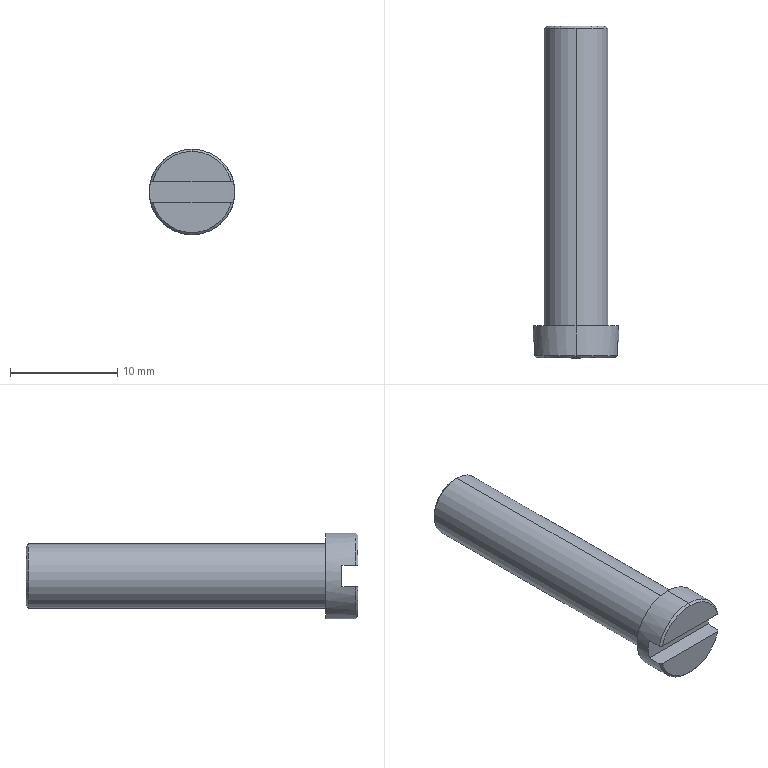Part | NX | features BREP 1 | 1 solid | 20 faces | box 8 x 31 x 8 mm | volume 879.904 mm3 | plane 7 | cone 7 | cylinder 6 | commonest cylinder face diameters 2.5 x2 6 x2 8 x2
STEP:
#1=CARTESIAN_POINT('',(3.873,1.5,1.));
#2=VERTEX_POINT('',#1);
#3=CARTESIAN_POINT('',(-3.873,1.5,1.));
#4=VERTEX_POINT('',#3);
#5=CARTESIAN_POINT('',(-4.,1.5,1.));
#6=DIRECTION('',(-1.,0.,0.));
#7=VECTOR('',#6,1000.);
#8=LINE('',#5,#7);
#9=EDGE_CURVE('',#2,#4,#8,.T.);
#10=ORIENTED_EDGE('',*,*,#9,.T.);
#11=CARTESIAN_POINT('',(-3.873,1.5,-1.));
#12=VERTEX_POINT('',#11);
#13=CARTESIAN_POINT('',(0.,1.5,0.));
#14=DIRECTION('',(0.,-1.,0.));
#15=DIRECTION('',(0.,0.,1.));
#16=AXIS2_PLACEMENT_3D('',#13,#14,#15);
#17=CIRCLE('',#16,4.);
#18=EDGE_CURVE('',#4,#12,#17,.T.);
#19=ORIENTED_EDGE('',*,*,#18,.T.);
#20=CARTESIAN_POINT('',(3.873,1.5,-1.));
#21=VERTEX_POINT('',#20);
#22=CARTESIAN_POINT('',(-4.,1.5,-1.));
#23=DIRECTION('',(1.,0.,0.));
#24=VECTOR('',#23,1000.);
#25=LINE('',#22,#24);
#26=EDGE_CURVE('',#12,#21,#25,.T.);
#27=ORIENTED_EDGE('',*,*,#26,.T.);
#28=CARTESIAN_POINT('',(0.,1.5,0.));
#29=DIRECTION('',(0.,-1.,0.));
#30=DIRECTION('',(0.,0.,1.));
#31=AXIS2_PLACEMENT_3D('',#28,#29,#30);
#32=CIRCLE('',#31,4.);
#33=EDGE_CURVE('',#21,#2,#32,.T.);
#34=ORIENTED_EDGE('',*,*,#33,.T.);
#35=EDGE_LOOP('',(#10,#19,#27,#34));
#36=FACE_BOUND('',#35,.T.);
#37=CARTESIAN_POINT('',(0.,1.5,0.));
#38=DIRECTION('',(0.,1.,0.));
#39=DIRECTION('',(0.,0.,1.));
#40=AXIS2_PLACEMENT_3D('',#37,#38,#39);
#41=PLANE('',#40);
#42=ADVANCED_FACE('',(#36),#41,.F.);
#43=CARTESIAN_POINT('',(3.873,0.2,1.));
#44=VERTEX_POINT('',#43);
#45=CARTESIAN_POINT('',(3.873,0.,1.));
#46=DIRECTION('',(0.,-1.,0.));
#47=VECTOR('',#46,1000.);
#48=LINE('',#45,#47);
#49=EDGE_CURVE('',#2,#44,#48,.T.);
#50=ORIENTED_EDGE('',*,*,#49,.T.);
#51=CARTESIAN_POINT('',(3.666,0.,1.));
#52=VERTEX_POINT('',#51);
#53=CARTESIAN_POINT('',(3.873,0.2,1.));
#54=CARTESIAN_POINT('',(3.804,0.1333,1.));
#55=CARTESIAN_POINT('',(3.735,0.0666,1.));
#56=CARTESIAN_POINT('',(3.666,0.,1.));
#57=B_SPLINE_CURVE_WITH_KNOTS('',3,(#53,#54,#55,#56),.UNSPECIFIED.,.F.,.F.,(4,4),(0.00684,0.007128),.UNSPECIFIED.);
#58=EDGE_CURVE('',#44,#52,#57,.T.);
#59=ORIENTED_EDGE('',*,*,#58,.T.);
#60=CARTESIAN_POINT('',(-3.666,0.,1.));
#61=VERTEX_POINT('',#60);
#62=CARTESIAN_POINT('',(-4.,0.,1.));
#63=DIRECTION('',(-1.,0.,0.));
#64=VECTOR('',#63,1000.);
#65=LINE('',#62,#64);
#66=EDGE_CURVE('',#52,#61,#65,.T.);
#67=ORIENTED_EDGE('',*,*,#66,.T.);
#68=CARTESIAN_POINT('',(-3.873,0.2,1.));
#69=VERTEX_POINT('',#68);
#70=CARTESIAN_POINT('',(-3.666,0.,1.));
#71=CARTESIAN_POINT('',(-3.735,0.0666,1.));
#72=CARTESIAN_POINT('',(-3.804,0.1333,1.));
#73=CARTESIAN_POINT('',(-3.873,0.2,1.));
#74=B_SPLINE_CURVE_WITH_KNOTS('',3,(#70,#71,#72,#73),.UNSPECIFIED.,.F.,.F.,(4,4),(0.01642,0.01671),.UNSPECIFIED.);
#75=EDGE_CURVE('',#61,#69,#74,.T.);
#76=ORIENTED_EDGE('',*,*,#75,.T.);
#77=CARTESIAN_POINT('',(-3.873,0.,1.));
#78=DIRECTION('',(0.,1.,0.));
#79=VECTOR('',#78,1000.);
#80=LINE('',#77,#79);
#81=EDGE_CURVE('',#69,#4,#80,.T.);
#82=ORIENTED_EDGE('',*,*,#81,.T.);
#83=ORIENTED_EDGE('',*,*,#9,.F.);
#84=EDGE_LOOP('',(#50,#59,#67,#76,#82,#83));
#85=FACE_BOUND('',#84,.T.);
#86=CARTESIAN_POINT('',(-4.,1.5,1.));
#87=DIRECTION('',(0.,0.,1.));
#88=DIRECTION('',(1.,0.,0.));
#89=AXIS2_PLACEMENT_3D('',#86,#87,#88);
#90=PLANE('',#89);
#91=ADVANCED_FACE('',(#85),#90,.F.);
#92=CARTESIAN_POINT('',(-3.873,0.2,-1.));
#93=VERTEX_POINT('',#92);
#94=CARTESIAN_POINT('',(-3.873,0.,-1.));
#95=DIRECTION('',(0.,-1.,0.));
#96=VECTOR('',#95,1000.);
#97=LINE('',#94,#96);
#98=EDGE_CURVE('',#12,#93,#97,.T.);
#99=ORIENTED_EDGE('',*,*,#98,.T.);
#100=CARTESIAN_POINT('',(-3.666,0.,-1.));
#101=VERTEX_POINT('',#100);
#102=CARTESIAN_POINT('',(-3.873,0.2,-1.));
#103=CARTESIAN_POINT('',(-3.804,0.1333,-1.));
#104=CARTESIAN_POINT('',(-3.735,0.0666,-1.));
#105=CARTESIAN_POINT('',(-3.666,0.,-1.));
#106=B_SPLINE_CURVE_WITH_KNOTS('',3,(#102,#103,#104,#105),.UNSPECIFIED.,.F.,.F.,(4,4),(0.00684,0.007128),.UNSPECIFIED.);
#107=EDGE_CURVE('',#93,#101,#106,.T.);
#108=ORIENTED_EDGE('',*,*,#107,.T.);
#109=CARTESIAN_POINT('',(3.666,0.,-1.));
#110=VERTEX_POINT('',#109);
#111=CARTESIAN_POINT('',(-4.,0.,-1.));
#112=DIRECTION('',(1.,0.,0.));
#113=VECTOR('',#112,1000.);
#114=LINE('',#111,#113);
#115=EDGE_CURVE('',#101,#110,#114,.T.);
#116=ORIENTED_EDGE('',*,*,#115,.T.);
#117=CARTESIAN_POINT('',(3.873,0.2,-1.));
#118=VERTEX_POINT('',#117);
#119=CARTESIAN_POINT('',(3.666,0.,-1.));
#120=CARTESIAN_POINT('',(3.735,0.0666,-1.));
#121=CARTESIAN_POINT('',(3.804,0.1333,-1.));
#122=CARTESIAN_POINT('',(3.873,0.2,-1.));
#123=B_SPLINE_CURVE_WITH_KNOTS('',3,(#119,#120,#121,#122),.UNSPECIFIED.,.F.,.F.,(4,4),(0.01642,0.01671),.UNSPECIFIED.);
#124=EDGE_CURVE('',#110,#118,#123,.T.);
#125=ORIENTED_EDGE('',*,*,#124,.T.);
#126=CARTESIAN_POINT('',(3.873,0.,-1.));
#127=DIRECTION('',(0.,1.,0.));
#128=VECTOR('',#127,1000.);
#129=LINE('',#126,#128);
#130=EDGE_CURVE('',#118,#21,#129,.T.);
#131=ORIENTED_EDGE('',*,*,#130,.T.);
#132=ORIENTED_EDGE('',*,*,#26,.F.);
#133=EDGE_LOOP('',(#99,#108,#116,#125,#131,#132));
#134=FACE_BOUND('',#133,.T.);
#135=CARTESIAN_POINT('',(-4.,1.5,-1.));
#136=DIRECTION('',(0.,0.,-1.));
#137=DIRECTION('',(-1.,0.,0.));
#138=AXIS2_PLACEMENT_3D('',#135,#136,#137);
#139=PLANE('',#138);
#140=ADVANCED_FACE('',(#134),#139,.F.);
#141=CARTESIAN_POINT('',(0.,0.,3.8));
#142=VERTEX_POINT('',#141);
#143=CARTESIAN_POINT('',(0.,0.2,4.));
#144=VERTEX_POINT('',#143);
#145=CARTESIAN_POINT('',(0.,0.2,4.));
#146=DIRECTION('',(0.,0.7071,0.7071));
#147=VECTOR('',#146,1000.);
#148=LINE('',#145,#147);
#149=EDGE_CURVE('',#142,#144,#148,.T.);
#150=ORIENTED_EDGE('',*,*,#149,.F.);
#151=CARTESIAN_POINT('',(0.,0.,0.));
#152=DIRECTION('',(0.,-1.,0.));
#153=DIRECTION('',(0.,0.,-1.));
#154=AXIS2_PLACEMENT_3D('',#151,#152,#153);
#155=CIRCLE('',#154,3.8);
#156=EDGE_CURVE('',#52,#142,#155,.T.);
#157=ORIENTED_EDGE('',*,*,#156,.F.);
#158=ORIENTED_EDGE('',*,*,#58,.F.);
#159=CARTESIAN_POINT('',(0.,0.2,0.));
#160=DIRECTION('',(0.,1.,0.));
#161=DIRECTION('',(0.,0.,-1.));
#162=AXIS2_PLACEMENT_3D('',#159,#160,#161);
#163=CIRCLE('',#162,4.);
#164=EDGE_CURVE('',#144,#44,#163,.T.);
#165=ORIENTED_EDGE('',*,*,#164,.F.);
#166=EDGE_LOOP('',(#150,#157,#158,#165));
#167=FACE_BOUND('',#166,.T.);
#168=CARTESIAN_POINT('',(0.,0.2,0.));
#169=DIRECTION('',(0.,1.,0.));
#170=DIRECTION('',(0.,0.,1.));
#171=AXIS2_PLACEMENT_3D('',#168,#169,#170);
#172=CONICAL_SURFACE('',#171,4.,0.7854);
#173=ADVANCED_FACE('',(#167),#172,.T.);
#174=CARTESIAN_POINT('',(0.,31.,2.8));
#175=VERTEX_POINT('',#174);
#176=CARTESIAN_POINT('',(0.,30.8,3.));
#177=VERTEX_POINT('',#176);
#178=CARTESIAN_POINT('',(0.,31.,2.8));
#179=DIRECTION('',(0.,-0.7071,0.7071));
#180=VECTOR('',#179,1000.);
#181=LINE('',#178,#180);
#182=EDGE_CURVE('',#175,#177,#181,.T.);
#183=ORIENTED_EDGE('',*,*,#182,.F.);
#184=CARTESIAN_POINT('',(0.,31.,-2.8));
#185=VERTEX_POINT('',#184);
#186=CARTESIAN_POINT('',(0.,31.,0.));
#187=DIRECTION('',(0.,1.,0.));
#188=DIRECTION('',(0.,0.,1.));
#189=AXIS2_PLACEMENT_3D('',#186,#187,#188);
#190=CIRCLE('',#189,2.8);
#191=EDGE_CURVE('',#185,#175,#190,.T.);
#192=ORIENTED_EDGE('',*,*,#191,.F.);
#193=CARTESIAN_POINT('',(0.,30.8,-3.));
#194=VERTEX_POINT('',#193);
#195=CARTESIAN_POINT('',(0.,31.,-2.8));
#196=DIRECTION('',(0.,-0.7071,-0.7071));
#197=VECTOR('',#196,1000.);
#198=LINE('',#195,#197);
#199=EDGE_CURVE('',#185,#194,#198,.T.);
#200=ORIENTED_EDGE('',*,*,#199,.T.);
#201=CARTESIAN_POINT('',(0.,30.8,0.));
#202=DIRECTION('',(0.,-1.,0.));
#203=DIRECTION('',(0.,0.,1.));
#204=AXIS2_PLACEMENT_3D('',#201,#202,#203);
#205=CIRCLE('',#204,3.);
#206=EDGE_CURVE('',#177,#194,#205,.T.);
#207=ORIENTED_EDGE('',*,*,#206,.F.);
#208=EDGE_LOOP('',(#183,#192,#200,#207));
#209=FACE_BOUND('',#208,.T.);
#210=CARTESIAN_POINT('',(0.,31.,0.));
#211=DIRECTION('',(0.,-1.,0.));
#212=DIRECTION('',(0.,0.,-1.));
#213=AXIS2_PLACEMENT_3D('',#210,#211,#212);
#214=CONICAL_SURFACE('',#213,2.8,0.7854);
#215=ADVANCED_FACE('',(#209),#214,.T.);
#216=CARTESIAN_POINT('',(0.,31.,-1.25));
#217=VERTEX_POINT('',#216);
#218=CARTESIAN_POINT('',(0.,23.5,-1.25));
#219=VERTEX_POINT('',#218);
#220=CARTESIAN_POINT('',(0.,31.,-1.25));
#221=DIRECTION('',(0.,1.,0.));
#222=VECTOR('',#221,1000.);
#223=LINE('',#220,#222);
#224=EDGE_CURVE('',#217,#219,#223,.F.);
#225=ORIENTED_EDGE('',*,*,#224,.T.);
#226=CARTESIAN_POINT('',(0.,23.5,1.25));
#227=VERTEX_POINT('',#226);
#228=CARTESIAN_POINT('',(0.,23.5,0.));
#229=DIRECTION('',(0.,1.,0.));
#230=DIRECTION('',(0.,0.,1.));
#231=AXIS2_PLACEMENT_3D('',#228,#229,#230);
#232=CIRCLE('',#231,1.25);
#233=EDGE_CURVE('',#227,#219,#232,.T.);
#234=ORIENTED_EDGE('',*,*,#233,.F.);
#235=CARTESIAN_POINT('',(0.,31.,1.25));
#236=VERTEX_POINT('',#235);
#237=CARTESIAN_POINT('',(0.,31.,1.25));
#238=DIRECTION('',(0.,1.,0.));
#239=VECTOR('',#238,1000.);
#240=LINE('',#237,#239);
#241=EDGE_CURVE('',#236,#227,#240,.F.);
#242=ORIENTED_EDGE('',*,*,#241,.F.);
#243=CARTESIAN_POINT('',(0.,31.,0.));
#244=DIRECTION('',(0.,1.,0.));
#245=DIRECTION('',(0.,0.,1.));
#246=AXIS2_PLACEMENT_3D('',#243,#244,#245);
#247=CIRCLE('',#246,1.25);
#248=EDGE_CURVE('',#236,#217,#247,.T.);
#249=ORIENTED_EDGE('',*,*,#248,.T.);
#250=EDGE_LOOP('',(#225,#234,#242,#249));
#251=FACE_BOUND('',#250,.T.);
#252=CARTESIAN_POINT('',(0.,31.,0.));
#253=DIRECTION('',(0.,1.,0.));
#254=DIRECTION('',(0.,0.,1.));
#255=AXIS2_PLACEMENT_3D('',#252,#253,#254);
#256=CYLINDRICAL_SURFACE('',#255,1.25);
#257=ADVANCED_FACE('',(#251),#256,.F.);
#258=CARTESIAN_POINT('',(0.,22.749,0.));
#259=VERTEX_POINT('',#258);
#260=CARTESIAN_POINT('',(0.,23.5,-1.25));
#261=DIRECTION('',(0.,0.515,-0.8572));
#262=VECTOR('',#261,1000.);
#263=LINE('',#260,#262);
#264=EDGE_CURVE('',#259,#219,#263,.T.);
#265=ORIENTED_EDGE('',*,*,#264,.F.);
#266=CARTESIAN_POINT('',(0.,23.5,1.25));
#267=DIRECTION('',(0.,0.515,0.8572));
#268=VECTOR('',#267,1000.);
#269=LINE('',#266,#268);
#270=EDGE_CURVE('',#259,#227,#269,.T.);
#271=ORIENTED_EDGE('',*,*,#270,.T.);
#272=ORIENTED_EDGE('',*,*,#233,.T.);
#273=EDGE_LOOP('',(#265,#271,#272));
#274=FACE_BOUND('',#273,.T.);
#275=CARTESIAN_POINT('',(0.,23.5,0.));
#276=DIRECTION('',(0.,1.,0.));
#277=DIRECTION('',(0.,0.,1.));
#278=AXIS2_PLACEMENT_3D('',#275,#276,#277);
#279=CONICAL_SURFACE('',#278,1.25,1.03);
#280=ADVANCED_FACE('',(#274),#279,.F.);
#281=ORIENTED_EDGE('',*,*,#66,.F.);
#282=ORIENTED_EDGE('',*,*,#156,.T.);
#283=CARTESIAN_POINT('',(0.,0.,0.));
#284=DIRECTION('',(0.,-1.,0.));
#285=DIRECTION('',(0.,0.,-1.));
#286=AXIS2_PLACEMENT_3D('',#283,#284,#285);
#287=CIRCLE('',#286,3.8);
#288=EDGE_CURVE('',#142,#61,#287,.T.);
#289=ORIENTED_EDGE('',*,*,#288,.T.);
#290=EDGE_LOOP('',(#281,#282,#289));
#291=FACE_BOUND('',#290,.T.);
#292=CARTESIAN_POINT('',(0.,0.,0.));
#293=DIRECTION('',(0.,-1.,0.));
#294=DIRECTION('',(0.,0.,-1.));
#295=AXIS2_PLACEMENT_3D('',#292,#293,#294);
#296=PLANE('',#295);
#297=ADVANCED_FACE('',(#291),#296,.T.);
#298=CARTESIAN_POINT('',(0.,3.,-4.));
#299=VERTEX_POINT('',#298);
#300=CARTESIAN_POINT('',(0.,0.2,-4.));
#301=VERTEX_POINT('',#300);
#302=CARTESIAN_POINT('',(0.,0.,-4.));
#303=DIRECTION('',(0.,1.,0.));
#304=VECTOR('',#303,1000.);
#305=LINE('',#302,#304);
#306=EDGE_CURVE('',#299,#301,#305,.F.);
#307=ORIENTED_EDGE('',*,*,#306,.T.);
#308=CARTESIAN_POINT('',(0.,0.2,0.));
#309=DIRECTION('',(0.,1.,0.));
#310=DIRECTION('',(0.,0.,-1.));
#311=AXIS2_PLACEMENT_3D('',#308,#309,#310);
#312=CIRCLE('',#311,4.);
#313=EDGE_CURVE('',#301,#93,#312,.T.);
#314=ORIENTED_EDGE('',*,*,#313,.T.);
#315=ORIENTED_EDGE('',*,*,#98,.F.);
#316=ORIENTED_EDGE('',*,*,#18,.F.);
#317=ORIENTED_EDGE('',*,*,#81,.F.);
#318=CARTESIAN_POINT('',(0.,0.2,0.));
#319=DIRECTION('',(0.,1.,0.));
#320=DIRECTION('',(0.,0.,-1.));
#321=AXIS2_PLACEMENT_3D('',#318,#319,#320);
#322=CIRCLE('',#321,4.);
#323=EDGE_CURVE('',#69,#144,#322,.T.);
#324=ORIENTED_EDGE('',*,*,#323,.T.);
#325=CARTESIAN_POINT('',(0.,3.,4.));
#326=VERTEX_POINT('',#325);
#327=CARTESIAN_POINT('',(0.,0.,4.));
#328=DIRECTION('',(0.,1.,0.));
#329=VECTOR('',#328,1000.);
#330=LINE('',#327,#329);
#331=EDGE_CURVE('',#326,#144,#330,.F.);
#332=ORIENTED_EDGE('',*,*,#331,.F.);
#333=CARTESIAN_POINT('',(0.,3.,0.));
#334=DIRECTION('',(0.,1.,0.));
#335=DIRECTION('',(0.,0.,1.));
#336=AXIS2_PLACEMENT_3D('',#333,#334,#335);
#337=CIRCLE('',#336,4.);
#338=EDGE_CURVE('',#299,#326,#337,.T.);
#339=ORIENTED_EDGE('',*,*,#338,.F.);
#340=EDGE_LOOP('',(#307,#314,#315,#316,#317,#324,#332,#339));
#341=FACE_BOUND('',#340,.T.);
#342=CARTESIAN_POINT('',(0.,0.,0.));
#343=DIRECTION('',(0.,1.,0.));
#344=DIRECTION('',(0.,0.,1.));
#345=AXIS2_PLACEMENT_3D('',#342,#343,#344);
#346=CYLINDRICAL_SURFACE('',#345,4.);
#347=ADVANCED_FACE('',(#341),#346,.T.);
#348=CARTESIAN_POINT('',(0.,3.,3.));
#349=VERTEX_POINT('',#348);
#350=CARTESIAN_POINT('',(0.,3.,-3.));
#351=VERTEX_POINT('',#350);
#352=CARTESIAN_POINT('',(0.,3.,0.));
#353=DIRECTION('',(0.,1.,0.));
#354=DIRECTION('',(0.,0.,1.));
#355=AXIS2_PLACEMENT_3D('',#352,#353,#354);
#356=CIRCLE('',#355,3.);
#357=EDGE_CURVE('',#349,#351,#356,.T.);
#358=ORIENTED_EDGE('',*,*,#357,.F.);
#359=CARTESIAN_POINT('',(0.,3.,0.));
#360=DIRECTION('',(0.,1.,0.));
#361=DIRECTION('',(0.,0.,1.));
#362=AXIS2_PLACEMENT_3D('',#359,#360,#361);
#363=CIRCLE('',#362,3.);
#364=EDGE_CURVE('',#351,#349,#363,.T.);
#365=ORIENTED_EDGE('',*,*,#364,.F.);
#366=EDGE_LOOP('',(#358,#365));
#367=FACE_BOUND('',#366,.T.);
#368=CARTESIAN_POINT('',(0.,3.,0.));
#369=DIRECTION('',(0.,1.,0.));
#370=DIRECTION('',(0.,0.,1.));
#371=AXIS2_PLACEMENT_3D('',#368,#369,#370);
#372=CIRCLE('',#371,4.);
#373=EDGE_CURVE('',#326,#299,#372,.T.);
#374=ORIENTED_EDGE('',*,*,#373,.T.);
#375=ORIENTED_EDGE('',*,*,#338,.T.);
#376=EDGE_LOOP('',(#374,#375));
#377=FACE_BOUND('',#376,.T.);
#378=CARTESIAN_POINT('',(0.,3.,0.));
#379=DIRECTION('',(0.,1.,0.));
#380=DIRECTION('',(0.,0.,1.));
#381=AXIS2_PLACEMENT_3D('',#378,#379,#380);
#382=PLANE('',#381);
#383=ADVANCED_FACE('',(#367,#377),#382,.T.);
#384=CARTESIAN_POINT('',(0.,0.,-3.));
#385=DIRECTION('',(0.,1.,0.));
#386=VECTOR('',#385,1000.);
#387=LINE('',#384,#386);
#388=EDGE_CURVE('',#194,#351,#387,.F.);
#389=ORIENTED_EDGE('',*,*,#388,.T.);
#390=ORIENTED_EDGE('',*,*,#364,.T.);
#391=CARTESIAN_POINT('',(0.,0.,3.));
#392=DIRECTION('',(0.,1.,0.));
#393=VECTOR('',#392,1000.);
#394=LINE('',#391,#393);
#395=EDGE_CURVE('',#177,#349,#394,.F.);
#396=ORIENTED_EDGE('',*,*,#395,.F.);
#397=ORIENTED_EDGE('',*,*,#206,.T.);
#398=EDGE_LOOP('',(#389,#390,#396,#397));
#399=FACE_BOUND('',#398,.T.);
#400=CARTESIAN_POINT('',(0.,0.,0.));
#401=DIRECTION('',(0.,1.,0.));
#402=DIRECTION('',(0.,0.,1.));
#403=AXIS2_PLACEMENT_3D('',#400,#401,#402);
#404=CYLINDRICAL_SURFACE('',#403,3.);
#405=ADVANCED_FACE('',(#399),#404,.T.);
#406=ORIENTED_EDGE('',*,*,#248,.F.);
#407=CARTESIAN_POINT('',(0.,31.,0.));
#408=DIRECTION('',(0.,1.,0.));
#409=DIRECTION('',(0.,0.,1.));
#410=AXIS2_PLACEMENT_3D('',#407,#408,#409);
#411=CIRCLE('',#410,1.25);
#412=EDGE_CURVE('',#217,#236,#411,.T.);
#413=ORIENTED_EDGE('',*,*,#412,.F.);
#414=EDGE_LOOP('',(#406,#413));
#415=FACE_BOUND('',#414,.T.);
#416=ORIENTED_EDGE('',*,*,#191,.T.);
#417=CARTESIAN_POINT('',(0.,31.,0.));
#418=DIRECTION('',(0.,1.,0.));
#419=DIRECTION('',(0.,0.,1.));
#420=AXIS2_PLACEMENT_3D('',#417,#418,#419);
#421=CIRCLE('',#420,2.8);
#422=EDGE_CURVE('',#175,#185,#421,.T.);
#423=ORIENTED_EDGE('',*,*,#422,.T.);
#424=EDGE_LOOP('',(#416,#423));
#425=FACE_BOUND('',#424,.T.);
#426=CARTESIAN_POINT('',(0.,31.,0.));
#427=DIRECTION('',(0.,1.,0.));
#428=DIRECTION('',(0.,0.,1.));
#429=AXIS2_PLACEMENT_3D('',#426,#427,#428);
#430=PLANE('',#429);
#431=ADVANCED_FACE('',(#415,#425),#430,.T.);
#432=ORIENTED_EDGE('',*,*,#107,.F.);
#433=ORIENTED_EDGE('',*,*,#313,.F.);
#434=CARTESIAN_POINT('',(0.,0.2,0.));
#435=DIRECTION('',(0.,1.,0.));
#436=DIRECTION('',(0.,0.,-1.));
#437=AXIS2_PLACEMENT_3D('',#434,#435,#436);
#438=CIRCLE('',#437,4.);
#439=EDGE_CURVE('',#118,#301,#438,.T.);
#440=ORIENTED_EDGE('',*,*,#439,.F.);
#441=ORIENTED_EDGE('',*,*,#124,.F.);
#442=CARTESIAN_POINT('',(0.,0.,0.));
#443=DIRECTION('',(0.,-1.,0.));
#444=DIRECTION('',(0.,0.,-1.));
#445=AXIS2_PLACEMENT_3D('',#442,#443,#444);
#446=CIRCLE('',#445,3.8);
#447=EDGE_CURVE('',#101,#110,#446,.T.);
#448=ORIENTED_EDGE('',*,*,#447,.F.);
#449=EDGE_LOOP('',(#432,#433,#440,#441,#448));
#450=FACE_BOUND('',#449,.T.);
#451=CARTESIAN_POINT('',(0.,0.2,0.));
#452=DIRECTION('',(0.,1.,0.));
#453=DIRECTION('',(0.,0.,1.));
#454=AXIS2_PLACEMENT_3D('',#451,#452,#453);
#455=CONICAL_SURFACE('',#454,4.,0.7854);
#456=ADVANCED_FACE('',(#450),#455,.T.);
#457=ORIENTED_EDGE('',*,*,#115,.F.);
#458=ORIENTED_EDGE('',*,*,#447,.T.);
#459=EDGE_LOOP('',(#457,#458));
#460=FACE_BOUND('',#459,.T.);
#461=CARTESIAN_POINT('',(0.,0.,0.));
#462=DIRECTION('',(0.,-1.,0.));
#463=DIRECTION('',(0.,0.,-1.));
#464=AXIS2_PLACEMENT_3D('',#461,#462,#463);
#465=PLANE('',#464);
#466=ADVANCED_FACE('',(#460),#465,.T.);
#467=ORIENTED_EDGE('',*,*,#357,.T.);
#468=ORIENTED_EDGE('',*,*,#388,.F.);
#469=CARTESIAN_POINT('',(0.,30.8,0.));
#470=DIRECTION('',(0.,-1.,0.));
#471=DIRECTION('',(0.,0.,1.));
#472=AXIS2_PLACEMENT_3D('',#469,#470,#471);
#473=CIRCLE('',#472,3.);
#474=EDGE_CURVE('',#194,#177,#473,.T.);
#475=ORIENTED_EDGE('',*,*,#474,.T.);
#476=ORIENTED_EDGE('',*,*,#395,.T.);
#477=EDGE_LOOP('',(#467,#468,#475,#476));
#478=FACE_BOUND('',#477,.T.);
#479=CARTESIAN_POINT('',(0.,0.,0.));
#480=DIRECTION('',(0.,1.,0.));
#481=DIRECTION('',(0.,0.,1.));
#482=AXIS2_PLACEMENT_3D('',#479,#480,#481);
#483=CYLINDRICAL_SURFACE('',#482,3.);
#484=ADVANCED_FACE('',(#478),#483,.T.);
#485=ORIENTED_EDGE('',*,*,#439,.T.);
#486=ORIENTED_EDGE('',*,*,#306,.F.);
#487=ORIENTED_EDGE('',*,*,#373,.F.);
#488=ORIENTED_EDGE('',*,*,#331,.T.);
#489=ORIENTED_EDGE('',*,*,#164,.T.);
#490=ORIENTED_EDGE('',*,*,#49,.F.);
#491=ORIENTED_EDGE('',*,*,#33,.F.);
#492=ORIENTED_EDGE('',*,*,#130,.F.);
#493=EDGE_LOOP('',(#485,#486,#487,#488,#489,#490,#491,#492));
#494=FACE_BOUND('',#493,.T.);
#495=CARTESIAN_POINT('',(0.,0.,0.));
#496=DIRECTION('',(0.,1.,0.));
#497=DIRECTION('',(0.,0.,1.));
#498=AXIS2_PLACEMENT_3D('',#495,#496,#497);
#499=CYLINDRICAL_SURFACE('',#498,4.);
#500=ADVANCED_FACE('',(#494),#499,.T.);
#501=ORIENTED_EDGE('',*,*,#270,.F.);
#502=ORIENTED_EDGE('',*,*,#264,.T.);
#503=CARTESIAN_POINT('',(0.,23.5,0.));
#504=DIRECTION('',(0.,1.,0.));
#505=DIRECTION('',(0.,0.,1.));
#506=AXIS2_PLACEMENT_3D('',#503,#504,#505);
#507=CIRCLE('',#506,1.25);
#508=EDGE_CURVE('',#219,#227,#507,.T.);
#509=ORIENTED_EDGE('',*,*,#508,.T.);
#510=EDGE_LOOP('',(#501,#502,#509));
#511=FACE_BOUND('',#510,.T.);
#512=CARTESIAN_POINT('',(0.,23.5,0.));
#513=DIRECTION('',(0.,1.,0.));
#514=DIRECTION('',(0.,0.,1.));
#515=AXIS2_PLACEMENT_3D('',#512,#513,#514);
#516=CONICAL_SURFACE('',#515,1.25,1.03);
#517=ADVANCED_FACE('',(#511),#516,.F.);
#518=ORIENTED_EDGE('',*,*,#508,.F.);
#519=ORIENTED_EDGE('',*,*,#224,.F.);
#520=ORIENTED_EDGE('',*,*,#412,.T.);
#521=ORIENTED_EDGE('',*,*,#241,.T.);
#522=EDGE_LOOP('',(#518,#519,#520,#521));
#523=FACE_BOUND('',#522,.T.);
#524=CARTESIAN_POINT('',(0.,31.,0.));
#525=DIRECTION('',(0.,1.,0.));
#526=DIRECTION('',(0.,0.,1.));
#527=AXIS2_PLACEMENT_3D('',#524,#525,#526);
#528=CYLINDRICAL_SURFACE('',#527,1.25);
#529=ADVANCED_FACE('',(#523),#528,.F.);
#530=ORIENTED_EDGE('',*,*,#422,.F.);
#531=ORIENTED_EDGE('',*,*,#182,.T.);
#532=ORIENTED_EDGE('',*,*,#474,.F.);
#533=ORIENTED_EDGE('',*,*,#199,.F.);
#534=EDGE_LOOP('',(#530,#531,#532,#533));
#535=FACE_BOUND('',#534,.T.);
#536=CARTESIAN_POINT('',(0.,31.,0.));
#537=DIRECTION('',(0.,-1.,0.));
#538=DIRECTION('',(0.,0.,-1.));
#539=AXIS2_PLACEMENT_3D('',#536,#537,#538);
#540=CONICAL_SURFACE('',#539,2.8,0.7854);
#541=ADVANCED_FACE('',(#535),#540,.T.);
#542=ORIENTED_EDGE('',*,*,#288,.F.);
#543=ORIENTED_EDGE('',*,*,#149,.T.);
#544=ORIENTED_EDGE('',*,*,#323,.F.);
#545=ORIENTED_EDGE('',*,*,#75,.F.);
#546=EDGE_LOOP('',(#542,#543,#544,#545));
#547=FACE_BOUND('',#546,.T.);
#548=CARTESIAN_POINT('',(0.,0.2,0.));
#549=DIRECTION('',(0.,1.,0.));
#550=DIRECTION('',(0.,0.,1.));
#551=AXIS2_PLACEMENT_3D('',#548,#549,#550);
#552=CONICAL_SURFACE('',#551,4.,0.7854);
#553=ADVANCED_FACE('',(#547),#552,.T.);
#554=CLOSED_SHELL('',(#42,#91,#140,#173,#215,#257,#280,#297,#347,#383,#405,#431,#456,#466,#484,#500,#517,#529,#541,#553));
#555=MANIFOLD_SOLID_BREP('',#554);
#556=(LENGTH_UNIT()NAMED_UNIT(*)SI_UNIT(.MILLI.,.METRE.));
#557=UNCERTAINTY_MEASURE_WITH_UNIT(LENGTH_MEASURE(0.00001),#556,'','');
#558=(NAMED_UNIT(*)PLANE_ANGLE_UNIT()SI_UNIT($,.RADIAN.));
#559=(NAMED_UNIT(*)SI_UNIT($,.STERADIAN.)SOLID_ANGLE_UNIT());
#560=(GEOMETRIC_REPRESENTATION_CONTEXT(3)GLOBAL_UNCERTAINTY_ASSIGNED_CONTEXT((#557))GLOBAL_UNIT_ASSIGNED_CONTEXT((#556,#558,#559))REPRESENTATION_CONTEXT('',''));
#561=ADVANCED_BREP_SHAPE_REPRESENTATION('',(#555),#560);